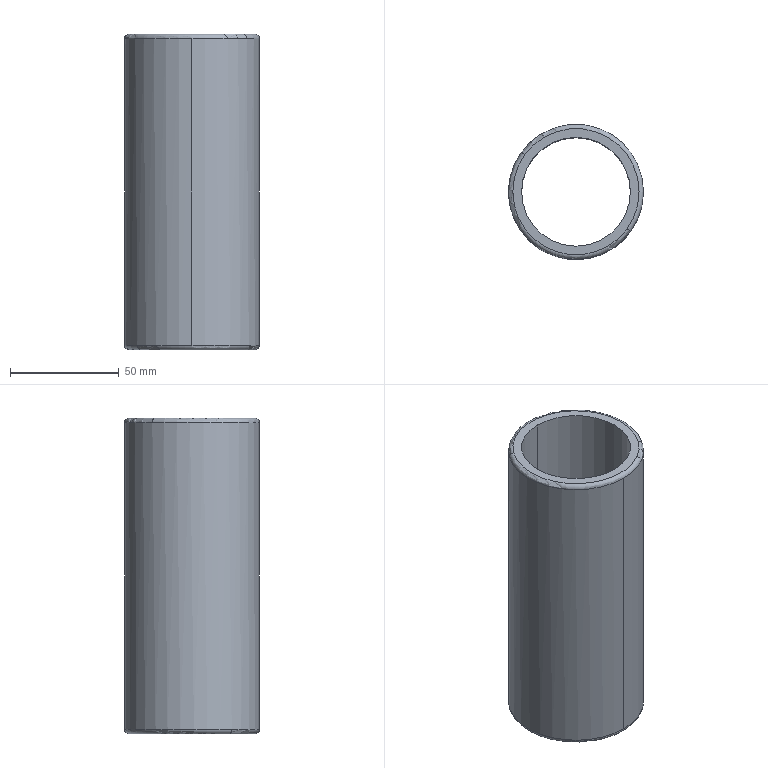Part | 1 solid | 10 faces | box 62 x 62 x 145 mm | volume 152729 mm3 | cylinder 4 | torus 4 | plane 2 | commonest cylinder face diameters 50 x2 62 x2
STEP:
#1=CARTESIAN_POINT('',(0.,0.,0.));
#2=DIRECTION('',(0.,0.,1.));
#3=DIRECTION('',(1.,0.,0.));
#4=AXIS2_PLACEMENT_3D('',#1,#2,#3);
#5=CARTESIAN_POINT('',(-480.,12.5,-188.55));
#6=VERTEX_POINT('',#5);
#7=CARTESIAN_POINT('',(-480.,12.5,-329.55));
#8=VERTEX_POINT('',#7);
#9=CARTESIAN_POINT('',(-480.,12.5,-188.55));
#10=DIRECTION('',(0.,0.,-1.));
#11=VECTOR('',#10,1.);
#12=LINE('',#9,#11);
#13=CARTESIAN_POINT('',(-480.,-18.5,-109.667));
#14=DIRECTION('',(0.,0.,-1.));
#15=DIRECTION('',(-1.,0.,0.));
#16=AXIS2_PLACEMENT_3D('',#13,#14,#15);
#17=CYLINDRICAL_SURFACE('',#16,31.);
#18=CARTESIAN_POINT('',(1.571,78.883));
#19=DIRECTION('',(0.,1.));
#20=VECTOR('',#19,1.);
#21=LINE('',#18,#20);
#22=(GEOMETRIC_REPRESENTATION_CONTEXT(2)PARAMETRIC_REPRESENTATION_CONTEXT()REPRESENTATION_CONTEXT('',''));
#23=DEFINITIONAL_REPRESENTATION('',(#21),#22);
#24=PCURVE('',#17,#23);
#25=CARTESIAN_POINT('',(-480.,-18.5,-109.667));
#26=DIRECTION('',(0.,0.,-1.));
#27=DIRECTION('',(1.,0.,0.));
#28=AXIS2_PLACEMENT_3D('',#25,#26,#27);
#29=CYLINDRICAL_SURFACE('',#28,31.);
#30=CARTESIAN_POINT('',(4.712,78.883));
#31=DIRECTION('',(0.,1.));
#32=VECTOR('',#31,1.);
#33=LINE('',#30,#32);
#34=(GEOMETRIC_REPRESENTATION_CONTEXT(2)PARAMETRIC_REPRESENTATION_CONTEXT()REPRESENTATION_CONTEXT('',''));
#35=DEFINITIONAL_REPRESENTATION('',(#33),#34);
#36=PCURVE('',#29,#35);
#37=SURFACE_CURVE('',#12,(#24,#36),.PCURVE_S1.);
#38=EDGE_CURVE('',#6,#8,#37,.T.);
#39=ORIENTED_EDGE('',*,*,#38,.F.);
#40=CARTESIAN_POINT('',(-454.92,-0.2787,-188.55));
#41=VERTEX_POINT('',#40);
#42=CARTESIAN_POINT('',(-480.,-18.5,-188.55));
#43=DIRECTION('',(0.,0.,-1.));
#44=DIRECTION('',(0.809,0.5878,0.));
#45=AXIS2_PLACEMENT_3D('',#42,#43,#44);
#46=CIRCLE('',#45,31.);
#47=CARTESIAN_POINT('',(-3.77,78.883));
#48=DIRECTION('',(1.,0.));
#49=VECTOR('',#48,1.);
#50=LINE('',#47,#49);
#51=(GEOMETRIC_REPRESENTATION_CONTEXT(2)PARAMETRIC_REPRESENTATION_CONTEXT()REPRESENTATION_CONTEXT('',''));
#52=DEFINITIONAL_REPRESENTATION('',(#50),#51);
#53=PCURVE('',#17,#52);
#54=CARTESIAN_POINT('',(-480.,-18.5,-188.55));
#55=DIRECTION('',(0.,0.,1.));
#56=DIRECTION('',(-0.5878,-0.809,0.));
#57=AXIS2_PLACEMENT_3D('',#54,#55,#56);
#58=TOROIDAL_SURFACE('',#57,29.,2.);
#59=CARTESIAN_POINT('',(9.111,0.));
#60=DIRECTION('',(-1.,0.));
#61=VECTOR('',#60,1.);
#62=LINE('',#59,#61);
#63=(GEOMETRIC_REPRESENTATION_CONTEXT(2)PARAMETRIC_REPRESENTATION_CONTEXT()REPRESENTATION_CONTEXT('',''));
#64=DEFINITIONAL_REPRESENTATION('',(#62),#63);
#65=PCURVE('',#58,#64);
#66=SURFACE_CURVE('',#46,(#53,#65),.PCURVE_S1.);
#67=EDGE_CURVE('',#6,#41,#66,.T.);
#68=ORIENTED_EDGE('',*,*,#67,.T.);
#69=CARTESIAN_POINT('',(-454.92,-36.721,-188.55));
#70=VERTEX_POINT('',#69);
#71=CARTESIAN_POINT('',(-480.,-18.5,-188.55));
#72=DIRECTION('',(0.,0.,-1.));
#73=DIRECTION('',(0.809,0.5878,0.));
#74=AXIS2_PLACEMENT_3D('',#71,#72,#73);
#75=CIRCLE('',#74,31.);
#76=CARTESIAN_POINT('',(2.513,78.883));
#77=DIRECTION('',(1.,0.));
#78=VECTOR('',#77,1.);
#79=LINE('',#76,#78);
#80=(GEOMETRIC_REPRESENTATION_CONTEXT(2)PARAMETRIC_REPRESENTATION_CONTEXT()REPRESENTATION_CONTEXT('',''));
#81=DEFINITIONAL_REPRESENTATION('',(#79),#80);
#82=PCURVE('',#17,#81);
#83=CARTESIAN_POINT('',(2.827,0.));
#84=DIRECTION('',(-1.,0.));
#85=VECTOR('',#84,1.);
#86=LINE('',#83,#85);
#87=(GEOMETRIC_REPRESENTATION_CONTEXT(2)PARAMETRIC_REPRESENTATION_CONTEXT()REPRESENTATION_CONTEXT('',''));
#88=DEFINITIONAL_REPRESENTATION('',(#86),#87);
#89=PCURVE('',#58,#88);
#90=SURFACE_CURVE('',#75,(#82,#89),.PCURVE_S1.);
#91=EDGE_CURVE('',#41,#70,#90,.T.);
#92=ORIENTED_EDGE('',*,*,#91,.T.);
#93=CARTESIAN_POINT('',(-480.,-49.5,-188.55));
#94=VERTEX_POINT('',#93);
#95=CARTESIAN_POINT('',(-480.,-18.5,-188.55));
#96=DIRECTION('',(0.,0.,-1.));
#97=DIRECTION('',(0.809,0.5878,0.));
#98=AXIS2_PLACEMENT_3D('',#95,#96,#97);
#99=CIRCLE('',#98,31.);
#100=CARTESIAN_POINT('',(2.513,78.883));
#101=DIRECTION('',(1.,0.));
#102=VECTOR('',#101,1.);
#103=LINE('',#100,#102);
#104=(GEOMETRIC_REPRESENTATION_CONTEXT(2)PARAMETRIC_REPRESENTATION_CONTEXT()REPRESENTATION_CONTEXT('',''));
#105=DEFINITIONAL_REPRESENTATION('',(#103),#104);
#106=PCURVE('',#17,#105);
#107=CARTESIAN_POINT('',(-480.,-18.5,-188.55));
#108=DIRECTION('',(0.,0.,1.));
#109=DIRECTION('',(0.5878,0.809,0.));
#110=AXIS2_PLACEMENT_3D('',#107,#108,#109);
#111=TOROIDAL_SURFACE('',#110,29.,2.);
#112=CARTESIAN_POINT('',(5.969,0.));
#113=DIRECTION('',(-1.,0.));
#114=VECTOR('',#113,1.);
#115=LINE('',#112,#114);
#116=(GEOMETRIC_REPRESENTATION_CONTEXT(2)PARAMETRIC_REPRESENTATION_CONTEXT()REPRESENTATION_CONTEXT('',''));
#117=DEFINITIONAL_REPRESENTATION('',(#115),#116);
#118=PCURVE('',#111,#117);
#119=SURFACE_CURVE('',#99,(#106,#118),.PCURVE_S1.);
#120=EDGE_CURVE('',#70,#94,#119,.T.);
#121=ORIENTED_EDGE('',*,*,#120,.T.);
#122=CARTESIAN_POINT('',(-480.,-49.5,-329.55));
#123=VERTEX_POINT('',#122);
#124=CARTESIAN_POINT('',(-480.,-49.5,-188.55));
#125=DIRECTION('',(0.,0.,-1.));
#126=VECTOR('',#125,1.);
#127=LINE('',#124,#126);
#128=CARTESIAN_POINT('',(4.712,78.883));
#129=DIRECTION('',(0.,1.));
#130=VECTOR('',#129,1.);
#131=LINE('',#128,#130);
#132=(GEOMETRIC_REPRESENTATION_CONTEXT(2)PARAMETRIC_REPRESENTATION_CONTEXT()REPRESENTATION_CONTEXT('',''));
#133=DEFINITIONAL_REPRESENTATION('',(#131),#132);
#134=PCURVE('',#17,#133);
#135=CARTESIAN_POINT('',(1.571,78.883));
#136=DIRECTION('',(0.,1.));
#137=VECTOR('',#136,1.);
#138=LINE('',#135,#137);
#139=(GEOMETRIC_REPRESENTATION_CONTEXT(2)PARAMETRIC_REPRESENTATION_CONTEXT()REPRESENTATION_CONTEXT('',''));
#140=DEFINITIONAL_REPRESENTATION('',(#138),#139);
#141=PCURVE('',#29,#140);
#142=SURFACE_CURVE('',#127,(#134,#141),.PCURVE_S1.);
#143=EDGE_CURVE('',#94,#123,#142,.T.);
#144=ORIENTED_EDGE('',*,*,#143,.T.);
#145=CARTESIAN_POINT('',(-454.92,-0.2787,-329.55));
#146=VERTEX_POINT('',#145);
#147=CARTESIAN_POINT('',(-480.,-18.5,-329.55));
#148=DIRECTION('',(0.,0.,-1.));
#149=DIRECTION('',(0.,-1.,0.));
#150=AXIS2_PLACEMENT_3D('',#147,#148,#149);
#151=CIRCLE('',#150,31.);
#152=CARTESIAN_POINT('',(-1.571,219.883));
#153=DIRECTION('',(1.,0.));
#154=VECTOR('',#153,1.);
#155=LINE('',#152,#154);
#156=(GEOMETRIC_REPRESENTATION_CONTEXT(2)PARAMETRIC_REPRESENTATION_CONTEXT()REPRESENTATION_CONTEXT('',''));
#157=DEFINITIONAL_REPRESENTATION('',(#155),#156);
#158=PCURVE('',#17,#157);
#159=CARTESIAN_POINT('',(-480.,-18.5,-329.55));
#160=DIRECTION('',(0.,0.,-1.));
#161=DIRECTION('',(-0.5878,0.809,0.));
#162=AXIS2_PLACEMENT_3D('',#159,#160,#161);
#163=TOROIDAL_SURFACE('',#162,29.,2.);
#164=CARTESIAN_POINT('',(-2.513,0.));
#165=DIRECTION('',(1.,0.));
#166=VECTOR('',#165,1.);
#167=LINE('',#164,#166);
#168=(GEOMETRIC_REPRESENTATION_CONTEXT(2)PARAMETRIC_REPRESENTATION_CONTEXT()REPRESENTATION_CONTEXT('',''));
#169=DEFINITIONAL_REPRESENTATION('',(#167),#168);
#170=PCURVE('',#163,#169);
#171=SURFACE_CURVE('',#151,(#158,#170),.PCURVE_S1.);
#172=EDGE_CURVE('',#146,#123,#171,.T.);
#173=ORIENTED_EDGE('',*,*,#172,.F.);
#174=CARTESIAN_POINT('',(-480.,-18.5,-329.55));
#175=DIRECTION('',(0.,0.,-1.));
#176=DIRECTION('',(0.,-1.,0.));
#177=AXIS2_PLACEMENT_3D('',#174,#175,#176);
#178=CIRCLE('',#177,31.);
#179=CARTESIAN_POINT('',(-1.571,219.883));
#180=DIRECTION('',(1.,0.));
#181=VECTOR('',#180,1.);
#182=LINE('',#179,#181);
#183=(GEOMETRIC_REPRESENTATION_CONTEXT(2)PARAMETRIC_REPRESENTATION_CONTEXT()REPRESENTATION_CONTEXT('',''));
#184=DEFINITIONAL_REPRESENTATION('',(#182),#183);
#185=PCURVE('',#17,#184);
#186=CARTESIAN_POINT('',(-480.,-18.5,-329.55));
#187=DIRECTION('',(0.,0.,-1.));
#188=DIRECTION('',(0.5878,-0.809,0.));
#189=AXIS2_PLACEMENT_3D('',#186,#187,#188);
#190=TOROIDAL_SURFACE('',#189,29.,2.);
#191=CARTESIAN_POINT('',(0.6283,0.));
#192=DIRECTION('',(1.,0.));
#193=VECTOR('',#192,1.);
#194=LINE('',#191,#193);
#195=(GEOMETRIC_REPRESENTATION_CONTEXT(2)PARAMETRIC_REPRESENTATION_CONTEXT()REPRESENTATION_CONTEXT('',''));
#196=DEFINITIONAL_REPRESENTATION('',(#194),#195);
#197=PCURVE('',#190,#196);
#198=SURFACE_CURVE('',#178,(#185,#197),.PCURVE_S1.);
#199=EDGE_CURVE('',#8,#146,#198,.T.);
#200=ORIENTED_EDGE('',*,*,#199,.F.);
#201=EDGE_LOOP('',(#39,#68,#92,#121,#144,#173,#200));
#202=FACE_BOUND('',#201,.T.);
#203=ADVANCED_FACE('',(#202),#17,.T.);
#204=CARTESIAN_POINT('',(-456.539,-35.546,-186.55));
#205=VERTEX_POINT('',#204);
#206=CARTESIAN_POINT('',(-456.539,-35.546,-188.55));
#207=DIRECTION('',(0.5878,0.809,0.));
#208=DIRECTION('',(0.,0.,1.));
#209=AXIS2_PLACEMENT_3D('',#206,#207,#208);
#210=CIRCLE('',#209,2.);
#211=CARTESIAN_POINT('',(1.571,1.571));
#212=DIRECTION('',(0.,-1.));
#213=VECTOR('',#212,1.);
#214=LINE('',#211,#213);
#215=(GEOMETRIC_REPRESENTATION_CONTEXT(2)PARAMETRIC_REPRESENTATION_CONTEXT()REPRESENTATION_CONTEXT('',''));
#216=DEFINITIONAL_REPRESENTATION('',(#214),#215);
#217=PCURVE('',#58,#216);
#218=CARTESIAN_POINT('',(4.712,1.571));
#219=DIRECTION('',(0.,-1.));
#220=VECTOR('',#219,1.);
#221=LINE('',#218,#220);
#222=(GEOMETRIC_REPRESENTATION_CONTEXT(2)PARAMETRIC_REPRESENTATION_CONTEXT()REPRESENTATION_CONTEXT('',''));
#223=DEFINITIONAL_REPRESENTATION('',(#221),#222);
#224=PCURVE('',#111,#223);
#225=SURFACE_CURVE('',#210,(#217,#224),.PCURVE_S1.);
#226=EDGE_CURVE('',#205,#70,#225,.T.);
#227=ORIENTED_EDGE('',*,*,#226,.T.);
#228=ORIENTED_EDGE('',*,*,#91,.F.);
#229=ORIENTED_EDGE('',*,*,#67,.F.);
#230=CARTESIAN_POINT('',(-505.08,-0.2787,-188.55));
#231=VERTEX_POINT('',#230);
#232=CARTESIAN_POINT('',(-480.,-18.5,-188.55));
#233=DIRECTION('',(0.,0.,-1.));
#234=DIRECTION('',(0.809,0.5878,0.));
#235=AXIS2_PLACEMENT_3D('',#232,#233,#234);
#236=CIRCLE('',#235,31.);
#237=CARTESIAN_POINT('',(9.111,0.));
#238=DIRECTION('',(-1.,0.));
#239=VECTOR('',#238,1.);
#240=LINE('',#237,#239);
#241=(GEOMETRIC_REPRESENTATION_CONTEXT(2)PARAMETRIC_REPRESENTATION_CONTEXT()REPRESENTATION_CONTEXT('',''));
#242=DEFINITIONAL_REPRESENTATION('',(#240),#241);
#243=PCURVE('',#58,#242);
#244=CARTESIAN_POINT('',(-0.6283,78.883));
#245=DIRECTION('',(1.,0.));
#246=VECTOR('',#245,1.);
#247=LINE('',#244,#246);
#248=(GEOMETRIC_REPRESENTATION_CONTEXT(2)PARAMETRIC_REPRESENTATION_CONTEXT()REPRESENTATION_CONTEXT('',''));
#249=DEFINITIONAL_REPRESENTATION('',(#247),#248);
#250=PCURVE('',#29,#249);
#251=SURFACE_CURVE('',#236,(#243,#250),.PCURVE_S1.);
#252=EDGE_CURVE('',#231,#6,#251,.T.);
#253=ORIENTED_EDGE('',*,*,#252,.F.);
#254=CARTESIAN_POINT('',(-503.461,-1.454,-186.55));
#255=VERTEX_POINT('',#254);
#256=CARTESIAN_POINT('',(-503.461,-1.454,-188.55));
#257=DIRECTION('',(-0.5878,-0.809,0.));
#258=DIRECTION('',(0.,0.,1.));
#259=AXIS2_PLACEMENT_3D('',#256,#257,#258);
#260=CIRCLE('',#259,2.);
#261=CARTESIAN_POINT('',(4.712,1.571));
#262=DIRECTION('',(0.,-1.));
#263=VECTOR('',#262,1.);
#264=LINE('',#261,#263);
#265=(GEOMETRIC_REPRESENTATION_CONTEXT(2)PARAMETRIC_REPRESENTATION_CONTEXT()REPRESENTATION_CONTEXT('',''));
#266=DEFINITIONAL_REPRESENTATION('',(#264),#265);
#267=PCURVE('',#58,#266);
#268=CARTESIAN_POINT('',(1.571,1.571));
#269=DIRECTION('',(0.,-1.));
#270=VECTOR('',#269,1.);
#271=LINE('',#268,#270);
#272=(GEOMETRIC_REPRESENTATION_CONTEXT(2)PARAMETRIC_REPRESENTATION_CONTEXT()REPRESENTATION_CONTEXT('',''));
#273=DEFINITIONAL_REPRESENTATION('',(#271),#272);
#274=PCURVE('',#111,#273);
#275=SURFACE_CURVE('',#260,(#267,#274),.PCURVE_S1.);
#276=EDGE_CURVE('',#255,#231,#275,.T.);
#277=ORIENTED_EDGE('',*,*,#276,.F.);
#278=CARTESIAN_POINT('',(-456.539,-1.454,-186.55));
#279=VERTEX_POINT('',#278);
#280=CARTESIAN_POINT('',(-480.,-18.5,-186.55));
#281=DIRECTION('',(0.,0.,-1.));
#282=DIRECTION('',(0.809,0.5878,0.));
#283=AXIS2_PLACEMENT_3D('',#280,#281,#282);
#284=CIRCLE('',#283,29.);
#285=CARTESIAN_POINT('',(9.111,1.571));
#286=DIRECTION('',(-1.,0.));
#287=VECTOR('',#286,1.);
#288=LINE('',#285,#287);
#289=(GEOMETRIC_REPRESENTATION_CONTEXT(2)PARAMETRIC_REPRESENTATION_CONTEXT()REPRESENTATION_CONTEXT('',''));
#290=DEFINITIONAL_REPRESENTATION('',(#288),#289);
#291=PCURVE('',#58,#290);
#292=CARTESIAN_POINT('',(-440.743,-18.5,-186.55));
#293=DIRECTION('',(0.,0.,1.));
#294=DIRECTION('',(0.,1.,0.));
#295=AXIS2_PLACEMENT_3D('',#292,#293,#294);
#296=PLANE('',#295);
#297=CARTESIAN_POINT('',(17.046,15.795));
#298=CARTESIAN_POINT('',(-23.591,-13.729));
#299=CARTESIAN_POINT('',(-28.841,36.226));
#300=CARTESIAN_POINT('',(-34.092,86.18));
#301=CARTESIAN_POINT('',(11.795,65.75));
#302=CARTESIAN_POINT('',(57.682,45.32));
#303=CARTESIAN_POINT('',(17.046,15.795));
#304=(BOUNDED_CURVE()B_SPLINE_CURVE(2,(#297,#298,#299,#300,#301,#302,#303),.UNSPECIFIED.,.T.,.F.)B_SPLINE_CURVE_WITH_KNOTS((1,2,2,2,2,1),(-2.094,0.,2.094,4.189,6.283,8.378),.UNSPECIFIED.)CURVE()GEOMETRIC_REPRESENTATION_ITEM()RATIONAL_B_SPLINE_CURVE((1.,0.5,1.,0.5,1.,0.5,1.))REPRESENTATION_ITEM(''));
#305=(GEOMETRIC_REPRESENTATION_CONTEXT(2)PARAMETRIC_REPRESENTATION_CONTEXT()REPRESENTATION_CONTEXT('',''));
#306=DEFINITIONAL_REPRESENTATION('',(#304),#305);
#307=PCURVE('',#296,#306);
#308=SURFACE_CURVE('',#284,(#291,#307),.PCURVE_S1.);
#309=EDGE_CURVE('',#255,#279,#308,.T.);
#310=ORIENTED_EDGE('',*,*,#309,.T.);
#311=CARTESIAN_POINT('',(-480.,-18.5,-186.55));
#312=DIRECTION('',(0.,0.,-1.));
#313=DIRECTION('',(0.809,0.5878,0.));
#314=AXIS2_PLACEMENT_3D('',#311,#312,#313);
#315=CIRCLE('',#314,29.);
#316=CARTESIAN_POINT('',(2.827,1.571));
#317=DIRECTION('',(-1.,0.));
#318=VECTOR('',#317,1.);
#319=LINE('',#316,#318);
#320=(GEOMETRIC_REPRESENTATION_CONTEXT(2)PARAMETRIC_REPRESENTATION_CONTEXT()REPRESENTATION_CONTEXT('',''));
#321=DEFINITIONAL_REPRESENTATION('',(#319),#320);
#322=PCURVE('',#58,#321);
#323=CARTESIAN_POINT('',(17.046,15.795));
#324=CARTESIAN_POINT('',(-23.591,-13.729));
#325=CARTESIAN_POINT('',(-28.841,36.226));
#326=CARTESIAN_POINT('',(-34.092,86.18));
#327=CARTESIAN_POINT('',(11.795,65.75));
#328=CARTESIAN_POINT('',(57.682,45.32));
#329=CARTESIAN_POINT('',(17.046,15.795));
#330=(BOUNDED_CURVE()B_SPLINE_CURVE(2,(#323,#324,#325,#326,#327,#328,#329),.UNSPECIFIED.,.T.,.F.)B_SPLINE_CURVE_WITH_KNOTS((1,2,2,2,2,1),(-2.094,0.,2.094,4.189,6.283,8.378),.UNSPECIFIED.)CURVE()GEOMETRIC_REPRESENTATION_ITEM()RATIONAL_B_SPLINE_CURVE((1.,0.5,1.,0.5,1.,0.5,1.))REPRESENTATION_ITEM(''));
#331=(GEOMETRIC_REPRESENTATION_CONTEXT(2)PARAMETRIC_REPRESENTATION_CONTEXT()REPRESENTATION_CONTEXT('',''));
#332=DEFINITIONAL_REPRESENTATION('',(#330),#331);
#333=PCURVE('',#296,#332);
#334=SURFACE_CURVE('',#315,(#322,#333),.PCURVE_S1.);
#335=EDGE_CURVE('',#279,#205,#334,.T.);
#336=ORIENTED_EDGE('',*,*,#335,.T.);
#337=EDGE_LOOP('',(#227,#228,#229,#253,#277,#310,#336));
#338=FACE_BOUND('',#337,.T.);
#339=ADVANCED_FACE('',(#338),#58,.T.);
#340=CARTESIAN_POINT('',(-480.,-43.5,-186.55));
#341=VERTEX_POINT('',#340);
#342=CARTESIAN_POINT('',(-480.,6.5,-186.55));
#343=VERTEX_POINT('',#342);
#344=CARTESIAN_POINT('',(-480.,-18.5,-186.55));
#345=DIRECTION('',(0.,0.,-1.));
#346=DIRECTION('',(0.,-1.,0.));
#347=AXIS2_PLACEMENT_3D('',#344,#345,#346);
#348=CIRCLE('',#347,25.);
#349=CARTESIAN_POINT('',(-25.,39.257));
#350=CARTESIAN_POINT('',(-25.,82.558));
#351=CARTESIAN_POINT('',(12.5,60.908));
#352=CARTESIAN_POINT('',(50.,39.257));
#353=CARTESIAN_POINT('',(12.5,17.606));
#354=CARTESIAN_POINT('',(-25.,-4.044));
#355=CARTESIAN_POINT('',(-25.,39.257));
#356=(BOUNDED_CURVE()B_SPLINE_CURVE(2,(#349,#350,#351,#352,#353,#354,#355),.UNSPECIFIED.,.T.,.F.)B_SPLINE_CURVE_WITH_KNOTS((1,2,2,2,2,1),(-2.094,0.,2.094,4.189,6.283,8.378),.UNSPECIFIED.)CURVE()GEOMETRIC_REPRESENTATION_ITEM()RATIONAL_B_SPLINE_CURVE((1.,0.5,1.,0.5,1.,0.5,1.))REPRESENTATION_ITEM(''));
#357=(GEOMETRIC_REPRESENTATION_CONTEXT(2)PARAMETRIC_REPRESENTATION_CONTEXT()REPRESENTATION_CONTEXT('',''));
#358=DEFINITIONAL_REPRESENTATION('',(#356),#357);
#359=PCURVE('',#296,#358);
#360=CARTESIAN_POINT('',(-480.,-18.5,-109.667));
#361=DIRECTION('',(0.,0.,-1.));
#362=DIRECTION('',(1.,0.,0.));
#363=AXIS2_PLACEMENT_3D('',#360,#361,#362);
#364=CYLINDRICAL_SURFACE('',#363,25.);
#365=CARTESIAN_POINT('',(1.571,76.883));
#366=DIRECTION('',(1.,0.));
#367=VECTOR('',#366,1.);
#368=LINE('',#365,#367);
#369=(GEOMETRIC_REPRESENTATION_CONTEXT(2)PARAMETRIC_REPRESENTATION_CONTEXT()REPRESENTATION_CONTEXT('',''));
#370=DEFINITIONAL_REPRESENTATION('',(#368),#369);
#371=PCURVE('',#364,#370);
#372=SURFACE_CURVE('',#348,(#359,#371),.PCURVE_S1.);
#373=EDGE_CURVE('',#341,#343,#372,.T.);
#374=ORIENTED_EDGE('',*,*,#373,.T.);
#375=CARTESIAN_POINT('',(-480.,-18.5,-186.55));
#376=DIRECTION('',(0.,0.,-1.));
#377=DIRECTION('',(0.,-1.,0.));
#378=AXIS2_PLACEMENT_3D('',#375,#376,#377);
#379=CIRCLE('',#378,25.);
#380=CARTESIAN_POINT('',(-25.,39.257));
#381=CARTESIAN_POINT('',(-25.,82.558));
#382=CARTESIAN_POINT('',(12.5,60.908));
#383=CARTESIAN_POINT('',(50.,39.257));
#384=CARTESIAN_POINT('',(12.5,17.606));
#385=CARTESIAN_POINT('',(-25.,-4.044));
#386=CARTESIAN_POINT('',(-25.,39.257));
#387=(BOUNDED_CURVE()B_SPLINE_CURVE(2,(#380,#381,#382,#383,#384,#385,#386),.UNSPECIFIED.,.T.,.F.)B_SPLINE_CURVE_WITH_KNOTS((1,2,2,2,2,1),(-2.094,0.,2.094,4.189,6.283,8.378),.UNSPECIFIED.)CURVE()GEOMETRIC_REPRESENTATION_ITEM()RATIONAL_B_SPLINE_CURVE((1.,0.5,1.,0.5,1.,0.5,1.))REPRESENTATION_ITEM(''));
#388=(GEOMETRIC_REPRESENTATION_CONTEXT(2)PARAMETRIC_REPRESENTATION_CONTEXT()REPRESENTATION_CONTEXT('',''));
#389=DEFINITIONAL_REPRESENTATION('',(#387),#388);
#390=PCURVE('',#296,#389);
#391=CARTESIAN_POINT('',(-480.,-18.5,-109.667));
#392=DIRECTION('',(0.,0.,-1.));
#393=DIRECTION('',(-1.,0.,0.));
#394=AXIS2_PLACEMENT_3D('',#391,#392,#393);
#395=CYLINDRICAL_SURFACE('',#394,25.);
#396=CARTESIAN_POINT('',(-1.571,76.883));
#397=DIRECTION('',(1.,0.));
#398=VECTOR('',#397,1.);
#399=LINE('',#396,#398);
#400=(GEOMETRIC_REPRESENTATION_CONTEXT(2)PARAMETRIC_REPRESENTATION_CONTEXT()REPRESENTATION_CONTEXT('',''));
#401=DEFINITIONAL_REPRESENTATION('',(#399),#400);
#402=PCURVE('',#395,#401);
#403=SURFACE_CURVE('',#379,(#390,#402),.PCURVE_S1.);
#404=EDGE_CURVE('',#343,#341,#403,.T.);
#405=ORIENTED_EDGE('',*,*,#404,.T.);
#406=EDGE_LOOP('',(#374,#405));
#407=FACE_BOUND('',#406,.T.);
#408=ORIENTED_EDGE('',*,*,#309,.F.);
#409=CARTESIAN_POINT('',(-480.,-18.5,-186.55));
#410=DIRECTION('',(0.,0.,-1.));
#411=DIRECTION('',(0.809,0.5878,0.));
#412=AXIS2_PLACEMENT_3D('',#409,#410,#411);
#413=CIRCLE('',#412,29.);
#414=CARTESIAN_POINT('',(17.046,15.795));
#415=CARTESIAN_POINT('',(-23.591,-13.729));
#416=CARTESIAN_POINT('',(-28.841,36.226));
#417=CARTESIAN_POINT('',(-34.092,86.18));
#418=CARTESIAN_POINT('',(11.795,65.75));
#419=CARTESIAN_POINT('',(57.682,45.32));
#420=CARTESIAN_POINT('',(17.046,15.795));
#421=(BOUNDED_CURVE()B_SPLINE_CURVE(2,(#414,#415,#416,#417,#418,#419,#420),.UNSPECIFIED.,.T.,.F.)B_SPLINE_CURVE_WITH_KNOTS((1,2,2,2,2,1),(-2.094,0.,2.094,4.189,6.283,8.378),.UNSPECIFIED.)CURVE()GEOMETRIC_REPRESENTATION_ITEM()RATIONAL_B_SPLINE_CURVE((1.,0.5,1.,0.5,1.,0.5,1.))REPRESENTATION_ITEM(''));
#422=(GEOMETRIC_REPRESENTATION_CONTEXT(2)PARAMETRIC_REPRESENTATION_CONTEXT()REPRESENTATION_CONTEXT('',''));
#423=DEFINITIONAL_REPRESENTATION('',(#421),#422);
#424=PCURVE('',#296,#423);
#425=CARTESIAN_POINT('',(5.969,1.571));
#426=DIRECTION('',(-1.,0.));
#427=VECTOR('',#426,1.);
#428=LINE('',#425,#427);
#429=(GEOMETRIC_REPRESENTATION_CONTEXT(2)PARAMETRIC_REPRESENTATION_CONTEXT()REPRESENTATION_CONTEXT('',''));
#430=DEFINITIONAL_REPRESENTATION('',(#428),#429);
#431=PCURVE('',#111,#430);
#432=SURFACE_CURVE('',#413,(#424,#431),.PCURVE_S1.);
#433=EDGE_CURVE('',#205,#255,#432,.T.);
#434=ORIENTED_EDGE('',*,*,#433,.F.);
#435=ORIENTED_EDGE('',*,*,#335,.F.);
#436=EDGE_LOOP('',(#408,#434,#435));
#437=FACE_BOUND('',#436,.T.);
#438=ADVANCED_FACE('',(#407,#437),#296,.T.);
#439=ORIENTED_EDGE('',*,*,#404,.T.);
#440=CARTESIAN_POINT('',(-480.,-43.5,-331.55));
#441=VERTEX_POINT('',#440);
#442=CARTESIAN_POINT('',(-480.,-43.5,-186.55));
#443=DIRECTION('',(0.,0.,-1.));
#444=VECTOR('',#443,1.);
#445=LINE('',#442,#444);
#446=CARTESIAN_POINT('',(4.712,76.883));
#447=DIRECTION('',(0.,1.));
#448=VECTOR('',#447,1.);
#449=LINE('',#446,#448);
#450=(GEOMETRIC_REPRESENTATION_CONTEXT(2)PARAMETRIC_REPRESENTATION_CONTEXT()REPRESENTATION_CONTEXT('',''));
#451=DEFINITIONAL_REPRESENTATION('',(#449),#450);
#452=PCURVE('',#395,#451);
#453=CARTESIAN_POINT('',(1.571,76.883));
#454=DIRECTION('',(0.,1.));
#455=VECTOR('',#454,1.);
#456=LINE('',#453,#455);
#457=(GEOMETRIC_REPRESENTATION_CONTEXT(2)PARAMETRIC_REPRESENTATION_CONTEXT()REPRESENTATION_CONTEXT('',''));
#458=DEFINITIONAL_REPRESENTATION('',(#456),#457);
#459=PCURVE('',#364,#458);
#460=SURFACE_CURVE('',#445,(#452,#459),.PCURVE_S1.);
#461=EDGE_CURVE('',#341,#441,#460,.T.);
#462=ORIENTED_EDGE('',*,*,#461,.T.);
#463=CARTESIAN_POINT('',(-480.,6.5,-331.55));
#464=VERTEX_POINT('',#463);
#465=CARTESIAN_POINT('',(-480.,-18.5,-331.55));
#466=DIRECTION('',(0.,0.,-1.));
#467=DIRECTION('',(0.,-1.,0.));
#468=AXIS2_PLACEMENT_3D('',#465,#466,#467);
#469=CIRCLE('',#468,25.);
#470=CARTESIAN_POINT('',(-1.571,221.883));
#471=DIRECTION('',(1.,0.));
#472=VECTOR('',#471,1.);
#473=LINE('',#470,#472);
#474=(GEOMETRIC_REPRESENTATION_CONTEXT(2)PARAMETRIC_REPRESENTATION_CONTEXT()REPRESENTATION_CONTEXT('',''));
#475=DEFINITIONAL_REPRESENTATION('',(#473),#474);
#476=PCURVE('',#395,#475);
#477=CARTESIAN_POINT('',(-444.243,-18.5,-331.55));
#478=DIRECTION('',(0.,0.,-1.));
#479=DIRECTION('',(0.,-1.,0.));
#480=AXIS2_PLACEMENT_3D('',#477,#478,#479);
#481=PLANE('',#480);
#482=CARTESIAN_POINT('',(0.,35.757));
#483=DIRECTION('',(1.,0.));
#484=AXIS2_PLACEMENT_2D('',#482,#483);
#485=CIRCLE('',#484,25.);
#486=(GEOMETRIC_REPRESENTATION_CONTEXT(2)PARAMETRIC_REPRESENTATION_CONTEXT()REPRESENTATION_CONTEXT('',''));
#487=DEFINITIONAL_REPRESENTATION('',(#485),#486);
#488=PCURVE('',#481,#487);
#489=SURFACE_CURVE('',#469,(#476,#488),.PCURVE_S1.);
#490=EDGE_CURVE('',#464,#441,#489,.T.);
#491=ORIENTED_EDGE('',*,*,#490,.F.);
#492=CARTESIAN_POINT('',(-480.,6.5,-186.55));
#493=DIRECTION('',(0.,0.,-1.));
#494=VECTOR('',#493,1.);
#495=LINE('',#492,#494);
#496=CARTESIAN_POINT('',(1.571,76.883));
#497=DIRECTION('',(0.,1.));
#498=VECTOR('',#497,1.);
#499=LINE('',#496,#498);
#500=(GEOMETRIC_REPRESENTATION_CONTEXT(2)PARAMETRIC_REPRESENTATION_CONTEXT()REPRESENTATION_CONTEXT('',''));
#501=DEFINITIONAL_REPRESENTATION('',(#499),#500);
#502=PCURVE('',#395,#501);
#503=CARTESIAN_POINT('',(4.712,76.883));
#504=DIRECTION('',(0.,1.));
#505=VECTOR('',#504,1.);
#506=LINE('',#503,#505);
#507=(GEOMETRIC_REPRESENTATION_CONTEXT(2)PARAMETRIC_REPRESENTATION_CONTEXT()REPRESENTATION_CONTEXT('',''));
#508=DEFINITIONAL_REPRESENTATION('',(#506),#507);
#509=PCURVE('',#364,#508);
#510=SURFACE_CURVE('',#495,(#502,#509),.PCURVE_S1.);
#511=EDGE_CURVE('',#343,#464,#510,.T.);
#512=ORIENTED_EDGE('',*,*,#511,.F.);
#513=EDGE_LOOP('',(#439,#462,#491,#512));
#514=FACE_BOUND('',#513,.F.);
#515=ADVANCED_FACE('',(#514),#395,.F.);
#516=CARTESIAN_POINT('',(-503.461,-1.454,-331.55));
#517=VERTEX_POINT('',#516);
#518=CARTESIAN_POINT('',(-456.539,-1.454,-331.55));
#519=VERTEX_POINT('',#518);
#520=CARTESIAN_POINT('',(-480.,-18.5,-331.55));
#521=DIRECTION('',(0.,0.,-1.));
#522=DIRECTION('',(-0.809,0.5878,0.));
#523=AXIS2_PLACEMENT_3D('',#520,#521,#522);
#524=CIRCLE('',#523,29.);
#525=CARTESIAN_POINT('',(0.,35.757));
#526=DIRECTION('',(-0.5878,0.809));
#527=AXIS2_PLACEMENT_2D('',#525,#526);
#528=CIRCLE('',#527,29.);
#529=(GEOMETRIC_REPRESENTATION_CONTEXT(2)PARAMETRIC_REPRESENTATION_CONTEXT()REPRESENTATION_CONTEXT('',''));
#530=DEFINITIONAL_REPRESENTATION('',(#528),#529);
#531=PCURVE('',#481,#530);
#532=CARTESIAN_POINT('',(2.827,1.571));
#533=DIRECTION('',(1.,0.));
#534=VECTOR('',#533,1.);
#535=LINE('',#532,#534);
#536=(GEOMETRIC_REPRESENTATION_CONTEXT(2)PARAMETRIC_REPRESENTATION_CONTEXT()REPRESENTATION_CONTEXT('',''));
#537=DEFINITIONAL_REPRESENTATION('',(#535),#536);
#538=PCURVE('',#190,#537);
#539=SURFACE_CURVE('',#524,(#531,#538),.PCURVE_S1.);
#540=EDGE_CURVE('',#517,#519,#539,.T.);
#541=ORIENTED_EDGE('',*,*,#540,.T.);
#542=CARTESIAN_POINT('',(-503.461,-35.546,-331.55));
#543=VERTEX_POINT('',#542);
#544=CARTESIAN_POINT('',(-480.,-18.5,-331.55));
#545=DIRECTION('',(0.,0.,-1.));
#546=DIRECTION('',(-0.809,0.5878,0.));
#547=AXIS2_PLACEMENT_3D('',#544,#545,#546);
#548=CIRCLE('',#547,29.);
#549=CARTESIAN_POINT('',(0.,35.757));
#550=DIRECTION('',(-0.5878,0.809));
#551=AXIS2_PLACEMENT_2D('',#549,#550);
#552=CIRCLE('',#551,29.);
#553=(GEOMETRIC_REPRESENTATION_CONTEXT(2)PARAMETRIC_REPRESENTATION_CONTEXT()REPRESENTATION_CONTEXT('',''));
#554=DEFINITIONAL_REPRESENTATION('',(#552),#553);
#555=PCURVE('',#481,#554);
#556=CARTESIAN_POINT('',(-0.3142,1.571));
#557=DIRECTION('',(1.,0.));
#558=VECTOR('',#557,1.);
#559=LINE('',#556,#558);
#560=(GEOMETRIC_REPRESENTATION_CONTEXT(2)PARAMETRIC_REPRESENTATION_CONTEXT()REPRESENTATION_CONTEXT('',''));
#561=DEFINITIONAL_REPRESENTATION('',(#559),#560);
#562=PCURVE('',#163,#561);
#563=SURFACE_CURVE('',#548,(#555,#562),.PCURVE_S1.);
#564=EDGE_CURVE('',#519,#543,#563,.T.);
#565=ORIENTED_EDGE('',*,*,#564,.T.);
#566=CARTESIAN_POINT('',(-480.,-18.5,-331.55));
#567=DIRECTION('',(0.,0.,-1.));
#568=DIRECTION('',(-0.809,0.5878,0.));
#569=AXIS2_PLACEMENT_3D('',#566,#567,#568);
#570=CIRCLE('',#569,29.);
#571=CARTESIAN_POINT('',(0.,35.757));
#572=DIRECTION('',(-0.5878,0.809));
#573=AXIS2_PLACEMENT_2D('',#571,#572);
#574=CIRCLE('',#573,29.);
#575=(GEOMETRIC_REPRESENTATION_CONTEXT(2)PARAMETRIC_REPRESENTATION_CONTEXT()REPRESENTATION_CONTEXT('',''));
#576=DEFINITIONAL_REPRESENTATION('',(#574),#575);
#577=PCURVE('',#481,#576);
#578=CARTESIAN_POINT('',(-3.456,1.571));
#579=DIRECTION('',(1.,0.));
#580=VECTOR('',#579,1.);
#581=LINE('',#578,#580);
#582=(GEOMETRIC_REPRESENTATION_CONTEXT(2)PARAMETRIC_REPRESENTATION_CONTEXT()REPRESENTATION_CONTEXT('',''));
#583=DEFINITIONAL_REPRESENTATION('',(#581),#582);
#584=PCURVE('',#190,#583);
#585=SURFACE_CURVE('',#570,(#577,#584),.PCURVE_S1.);
#586=EDGE_CURVE('',#543,#517,#585,.T.);
#587=ORIENTED_EDGE('',*,*,#586,.T.);
#588=EDGE_LOOP('',(#541,#565,#587));
#589=FACE_BOUND('',#588,.T.);
#590=ORIENTED_EDGE('',*,*,#490,.F.);
#591=CARTESIAN_POINT('',(-480.,-18.5,-331.55));
#592=DIRECTION('',(0.,0.,-1.));
#593=DIRECTION('',(0.,-1.,0.));
#594=AXIS2_PLACEMENT_3D('',#591,#592,#593);
#595=CIRCLE('',#594,25.);
#596=CARTESIAN_POINT('',(0.,35.757));
#597=DIRECTION('',(1.,0.));
#598=AXIS2_PLACEMENT_2D('',#596,#597);
#599=CIRCLE('',#598,25.);
#600=(GEOMETRIC_REPRESENTATION_CONTEXT(2)PARAMETRIC_REPRESENTATION_CONTEXT()REPRESENTATION_CONTEXT('',''));
#601=DEFINITIONAL_REPRESENTATION('',(#599),#600);
#602=PCURVE('',#481,#601);
#603=CARTESIAN_POINT('',(1.571,221.883));
#604=DIRECTION('',(1.,0.));
#605=VECTOR('',#604,1.);
#606=LINE('',#603,#605);
#607=(GEOMETRIC_REPRESENTATION_CONTEXT(2)PARAMETRIC_REPRESENTATION_CONTEXT()REPRESENTATION_CONTEXT('',''));
#608=DEFINITIONAL_REPRESENTATION('',(#606),#607);
#609=PCURVE('',#364,#608);
#610=SURFACE_CURVE('',#595,(#602,#609),.PCURVE_S1.);
#611=EDGE_CURVE('',#441,#464,#610,.T.);
#612=ORIENTED_EDGE('',*,*,#611,.F.);
#613=EDGE_LOOP('',(#590,#612));
#614=FACE_BOUND('',#613,.T.);
#615=ADVANCED_FACE('',(#589,#614),#481,.T.);
#616=CARTESIAN_POINT('',(-505.08,-36.721,-329.55));
#617=VERTEX_POINT('',#616);
#618=CARTESIAN_POINT('',(-503.461,-35.546,-329.55));
#619=DIRECTION('',(-0.5878,0.809,0.));
#620=DIRECTION('',(0.,0.,-1.));
#621=AXIS2_PLACEMENT_3D('',#618,#619,#620);
#622=CIRCLE('',#621,2.);
#623=CARTESIAN_POINT('',(1.571,1.571));
#624=DIRECTION('',(0.,-1.));
#625=VECTOR('',#624,1.);
#626=LINE('',#623,#625);
#627=(GEOMETRIC_REPRESENTATION_CONTEXT(2)PARAMETRIC_REPRESENTATION_CONTEXT()REPRESENTATION_CONTEXT('',''));
#628=DEFINITIONAL_REPRESENTATION('',(#626),#627);
#629=PCURVE('',#190,#628);
#630=CARTESIAN_POINT('',(4.712,1.571));
#631=DIRECTION('',(0.,-1.));
#632=VECTOR('',#631,1.);
#633=LINE('',#630,#632);
#634=(GEOMETRIC_REPRESENTATION_CONTEXT(2)PARAMETRIC_REPRESENTATION_CONTEXT()REPRESENTATION_CONTEXT('',''));
#635=DEFINITIONAL_REPRESENTATION('',(#633),#634);
#636=PCURVE('',#163,#635);
#637=SURFACE_CURVE('',#622,(#629,#636),.PCURVE_S1.);
#638=EDGE_CURVE('',#543,#617,#637,.T.);
#639=ORIENTED_EDGE('',*,*,#638,.T.);
#640=CARTESIAN_POINT('',(-480.,-18.5,-329.55));
#641=DIRECTION('',(0.,0.,-1.));
#642=DIRECTION('',(0.,-1.,0.));
#643=AXIS2_PLACEMENT_3D('',#640,#641,#642);
#644=CIRCLE('',#643,31.);
#645=CARTESIAN_POINT('',(0.6283,0.));
#646=DIRECTION('',(1.,0.));
#647=VECTOR('',#646,1.);
#648=LINE('',#645,#647);
#649=(GEOMETRIC_REPRESENTATION_CONTEXT(2)PARAMETRIC_REPRESENTATION_CONTEXT()REPRESENTATION_CONTEXT('',''));
#650=DEFINITIONAL_REPRESENTATION('',(#648),#649);
#651=PCURVE('',#190,#650);
#652=CARTESIAN_POINT('',(1.571,219.883));
#653=DIRECTION('',(1.,0.));
#654=VECTOR('',#653,1.);
#655=LINE('',#652,#654);
#656=(GEOMETRIC_REPRESENTATION_CONTEXT(2)PARAMETRIC_REPRESENTATION_CONTEXT()REPRESENTATION_CONTEXT('',''));
#657=DEFINITIONAL_REPRESENTATION('',(#655),#656);
#658=PCURVE('',#29,#657);
#659=SURFACE_CURVE('',#644,(#651,#658),.PCURVE_S1.);
#660=EDGE_CURVE('',#617,#8,#659,.T.);
#661=ORIENTED_EDGE('',*,*,#660,.T.);
#662=ORIENTED_EDGE('',*,*,#199,.T.);
#663=CARTESIAN_POINT('',(-456.539,-1.454,-329.55));
#664=DIRECTION('',(0.5878,-0.809,0.));
#665=DIRECTION('',(0.,0.,-1.));
#666=AXIS2_PLACEMENT_3D('',#663,#664,#665);
#667=CIRCLE('',#666,2.);
#668=CARTESIAN_POINT('',(4.712,1.571));
#669=DIRECTION('',(0.,-1.));
#670=VECTOR('',#669,1.);
#671=LINE('',#668,#670);
#672=(GEOMETRIC_REPRESENTATION_CONTEXT(2)PARAMETRIC_REPRESENTATION_CONTEXT()REPRESENTATION_CONTEXT('',''));
#673=DEFINITIONAL_REPRESENTATION('',(#671),#672);
#674=PCURVE('',#190,#673);
#675=CARTESIAN_POINT('',(1.571,1.571));
#676=DIRECTION('',(0.,-1.));
#677=VECTOR('',#676,1.);
#678=LINE('',#675,#677);
#679=(GEOMETRIC_REPRESENTATION_CONTEXT(2)PARAMETRIC_REPRESENTATION_CONTEXT()REPRESENTATION_CONTEXT('',''));
#680=DEFINITIONAL_REPRESENTATION('',(#678),#679);
#681=PCURVE('',#163,#680);
#682=SURFACE_CURVE('',#667,(#674,#681),.PCURVE_S1.);
#683=EDGE_CURVE('',#519,#146,#682,.T.);
#684=ORIENTED_EDGE('',*,*,#683,.F.);
#685=ORIENTED_EDGE('',*,*,#540,.F.);
#686=ORIENTED_EDGE('',*,*,#586,.F.);
#687=EDGE_LOOP('',(#639,#661,#662,#684,#685,#686));
#688=FACE_BOUND('',#687,.T.);
#689=ADVANCED_FACE('',(#688),#190,.T.);
#690=ORIENTED_EDGE('',*,*,#38,.T.);
#691=ORIENTED_EDGE('',*,*,#660,.F.);
#692=CARTESIAN_POINT('',(-480.,-18.5,-329.55));
#693=DIRECTION('',(0.,0.,-1.));
#694=DIRECTION('',(0.,-1.,0.));
#695=AXIS2_PLACEMENT_3D('',#692,#693,#694);
#696=CIRCLE('',#695,31.);
#697=CARTESIAN_POINT('',(1.571,219.883));
#698=DIRECTION('',(1.,0.));
#699=VECTOR('',#698,1.);
#700=LINE('',#697,#699);
#701=(GEOMETRIC_REPRESENTATION_CONTEXT(2)PARAMETRIC_REPRESENTATION_CONTEXT()REPRESENTATION_CONTEXT('',''));
#702=DEFINITIONAL_REPRESENTATION('',(#700),#701);
#703=PCURVE('',#29,#702);
#704=CARTESIAN_POINT('',(3.77,0.));
#705=DIRECTION('',(1.,0.));
#706=VECTOR('',#705,1.);
#707=LINE('',#704,#706);
#708=(GEOMETRIC_REPRESENTATION_CONTEXT(2)PARAMETRIC_REPRESENTATION_CONTEXT()REPRESENTATION_CONTEXT('',''));
#709=DEFINITIONAL_REPRESENTATION('',(#707),#708);
#710=PCURVE('',#163,#709);
#711=SURFACE_CURVE('',#696,(#703,#710),.PCURVE_S1.);
#712=EDGE_CURVE('',#123,#617,#711,.T.);
#713=ORIENTED_EDGE('',*,*,#712,.F.);
#714=ORIENTED_EDGE('',*,*,#143,.F.);
#715=CARTESIAN_POINT('',(-480.,-18.5,-188.55));
#716=DIRECTION('',(0.,0.,-1.));
#717=DIRECTION('',(0.809,0.5878,0.));
#718=AXIS2_PLACEMENT_3D('',#715,#716,#717);
#719=CIRCLE('',#718,31.);
#720=CARTESIAN_POINT('',(-0.6283,78.883));
#721=DIRECTION('',(1.,0.));
#722=VECTOR('',#721,1.);
#723=LINE('',#720,#722);
#724=(GEOMETRIC_REPRESENTATION_CONTEXT(2)PARAMETRIC_REPRESENTATION_CONTEXT()REPRESENTATION_CONTEXT('',''));
#725=DEFINITIONAL_REPRESENTATION('',(#723),#724);
#726=PCURVE('',#29,#725);
#727=CARTESIAN_POINT('',(5.969,0.));
#728=DIRECTION('',(-1.,0.));
#729=VECTOR('',#728,1.);
#730=LINE('',#727,#729);
#731=(GEOMETRIC_REPRESENTATION_CONTEXT(2)PARAMETRIC_REPRESENTATION_CONTEXT()REPRESENTATION_CONTEXT('',''));
#732=DEFINITIONAL_REPRESENTATION('',(#730),#731);
#733=PCURVE('',#111,#732);
#734=SURFACE_CURVE('',#719,(#726,#733),.PCURVE_S1.);
#735=EDGE_CURVE('',#94,#231,#734,.T.);
#736=ORIENTED_EDGE('',*,*,#735,.T.);
#737=ORIENTED_EDGE('',*,*,#252,.T.);
#738=EDGE_LOOP('',(#690,#691,#713,#714,#736,#737));
#739=FACE_BOUND('',#738,.T.);
#740=ADVANCED_FACE('',(#739),#29,.T.);
#741=ORIENTED_EDGE('',*,*,#226,.F.);
#742=ORIENTED_EDGE('',*,*,#433,.T.);
#743=ORIENTED_EDGE('',*,*,#276,.T.);
#744=ORIENTED_EDGE('',*,*,#735,.F.);
#745=ORIENTED_EDGE('',*,*,#120,.F.);
#746=EDGE_LOOP('',(#741,#742,#743,#744,#745));
#747=FACE_BOUND('',#746,.T.);
#748=ADVANCED_FACE('',(#747),#111,.T.);
#749=ORIENTED_EDGE('',*,*,#611,.F.);
#750=ORIENTED_EDGE('',*,*,#461,.F.);
#751=ORIENTED_EDGE('',*,*,#373,.T.);
#752=ORIENTED_EDGE('',*,*,#511,.T.);
#753=EDGE_LOOP('',(#749,#750,#751,#752));
#754=FACE_BOUND('',#753,.F.);
#755=ADVANCED_FACE('',(#754),#364,.F.);
#756=ORIENTED_EDGE('',*,*,#638,.F.);
#757=ORIENTED_EDGE('',*,*,#564,.F.);
#758=ORIENTED_EDGE('',*,*,#683,.T.);
#759=ORIENTED_EDGE('',*,*,#172,.T.);
#760=ORIENTED_EDGE('',*,*,#712,.T.);
#761=EDGE_LOOP('',(#756,#757,#758,#759,#760));
#762=FACE_BOUND('',#761,.T.);
#763=ADVANCED_FACE('',(#762),#163,.T.);
#764=CLOSED_SHELL('',(#203,#339,#438,#515,#615,#689,#740,#748,#755,#763));
#765=MANIFOLD_SOLID_BREP('',#764);
#766=(LENGTH_UNIT()NAMED_UNIT(*)SI_UNIT(.MILLI.,.METRE.));
#767=UNCERTAINTY_MEASURE_WITH_UNIT(LENGTH_MEASURE(0.0000001),#766,'','');
#768=(NAMED_UNIT(*)PLANE_ANGLE_UNIT()SI_UNIT($,.RADIAN.));
#769=(NAMED_UNIT(*)SI_UNIT($,.STERADIAN.)SOLID_ANGLE_UNIT());
#770=(GEOMETRIC_REPRESENTATION_CONTEXT(3)GLOBAL_UNCERTAINTY_ASSIGNED_CONTEXT((#767))GLOBAL_UNIT_ASSIGNED_CONTEXT((#766,#768,#769))REPRESENTATION_CONTEXT('',''));
#771=ADVANCED_BREP_SHAPE_REPRESENTATION('',(#4,#765),#770);